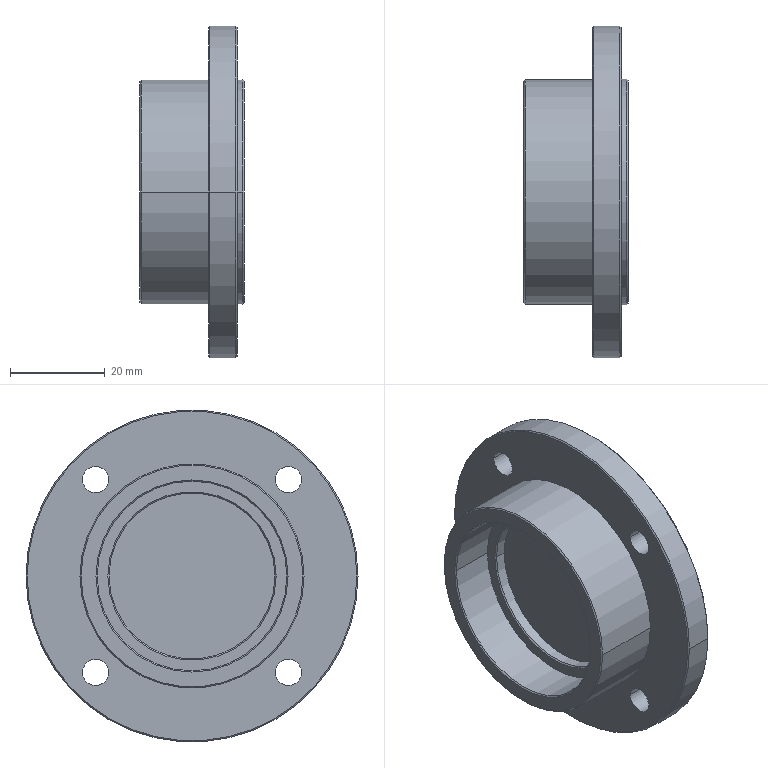Part | STEP file | 2026.6.15-Main Assembly图.sldasm-Part-104 | 1 solid | 36 faces | box 22 x 70 x 70 mm | volume 36230 mm3 | cylinder 18 | cone 12 | plane 6 | commonest cylinder face diameters 5.5 x8 35 x2 40 x2 47.25 x2 47.5 x2 70 x2
STEP:
#1=CARTESIAN_POINT('',(-1505.974,579.301,4296.167));
#2=VERTEX_POINT('',#1);
#3=CARTESIAN_POINT('',(-1505.974,539.301,4296.167));
#4=VERTEX_POINT('',#3);
#5=CARTESIAN_POINT('',(-1505.974,559.301,4296.167));
#6=DIRECTION('',(-1.,0.,0.));
#7=DIRECTION('',(0.,1.,0.));
#8=AXIS2_PLACEMENT_3D('',#5,#6,#7);
#9=CIRCLE('',#8,20.);
#10=EDGE_CURVE('',#2,#4,#9,.T.);
#11=ORIENTED_EDGE('',*,*,#10,.F.);
#12=CARTESIAN_POINT('',(-1506.224,579.551,4296.167));
#13=VERTEX_POINT('',#12);
#14=CARTESIAN_POINT('',(-1506.224,579.551,4296.167));
#15=DIRECTION('',(-0.7071,0.7071,0.));
#16=VECTOR('',#15,1000.);
#17=LINE('',#14,#16);
#18=EDGE_CURVE('',#2,#13,#17,.T.);
#19=ORIENTED_EDGE('',*,*,#18,.T.);
#20=CARTESIAN_POINT('',(-1506.224,539.051,4296.167));
#21=VERTEX_POINT('',#20);
#22=CARTESIAN_POINT('',(-1506.224,559.301,4296.167));
#23=DIRECTION('',(1.,0.,0.));
#24=DIRECTION('',(0.,0.,-1.));
#25=AXIS2_PLACEMENT_3D('',#22,#23,#24);
#26=CIRCLE('',#25,20.25);
#27=EDGE_CURVE('',#21,#13,#26,.T.);
#28=ORIENTED_EDGE('',*,*,#27,.F.);
#29=CARTESIAN_POINT('',(-1506.224,539.051,4296.167));
#30=DIRECTION('',(-0.7071,-0.7071,0.));
#31=VECTOR('',#30,1000.);
#32=LINE('',#29,#31);
#33=EDGE_CURVE('',#4,#21,#32,.T.);
#34=ORIENTED_EDGE('',*,*,#33,.F.);
#35=EDGE_LOOP('',(#11,#19,#28,#34));
#36=FACE_OUTER_BOUND('',#35,.T.);
#37=CARTESIAN_POINT('',(-1506.224,559.301,4296.167));
#38=DIRECTION('',(-1.,0.,0.));
#39=DIRECTION('',(0.,-1.,0.));
#40=AXIS2_PLACEMENT_3D('',#37,#38,#39);
#41=CONICAL_SURFACE('',#40,20.25,0.7854);
#42=ADVANCED_FACE('',(#36),#41,.F.);
#43=CARTESIAN_POINT('',(-1506.224,535.926,4296.167));
#44=VERTEX_POINT('',#43);
#45=CARTESIAN_POINT('',(-1506.224,582.676,4296.167));
#46=VERTEX_POINT('',#45);
#47=CARTESIAN_POINT('',(-1506.224,559.301,4296.167));
#48=DIRECTION('',(-1.,0.,0.));
#49=DIRECTION('',(0.,0.,-1.));
#50=AXIS2_PLACEMENT_3D('',#47,#48,#49);
#51=CIRCLE('',#50,23.375);
#52=EDGE_CURVE('',#44,#46,#51,.T.);
#53=ORIENTED_EDGE('',*,*,#52,.F.);
#54=CARTESIAN_POINT('',(-1505.974,535.676,4296.167));
#55=VERTEX_POINT('',#54);
#56=CARTESIAN_POINT('',(-1505.974,535.676,4296.167));
#57=DIRECTION('',(0.7071,-0.7071,0.));
#58=VECTOR('',#57,1000.);
#59=LINE('',#56,#58);
#60=EDGE_CURVE('',#44,#55,#59,.T.);
#61=ORIENTED_EDGE('',*,*,#60,.T.);
#62=CARTESIAN_POINT('',(-1505.974,582.926,4296.167));
#63=VERTEX_POINT('',#62);
#64=CARTESIAN_POINT('',(-1505.974,559.301,4296.167));
#65=DIRECTION('',(1.,0.,0.));
#66=DIRECTION('',(0.,1.,0.));
#67=AXIS2_PLACEMENT_3D('',#64,#65,#66);
#68=CIRCLE('',#67,23.625);
#69=EDGE_CURVE('',#63,#55,#68,.T.);
#70=ORIENTED_EDGE('',*,*,#69,.F.);
#71=CARTESIAN_POINT('',(-1505.974,582.926,4296.167));
#72=DIRECTION('',(0.7071,0.7071,0.));
#73=VECTOR('',#72,1000.);
#74=LINE('',#71,#73);
#75=EDGE_CURVE('',#46,#63,#74,.T.);
#76=ORIENTED_EDGE('',*,*,#75,.F.);
#77=EDGE_LOOP('',(#53,#61,#70,#76));
#78=FACE_OUTER_BOUND('',#77,.T.);
#79=CARTESIAN_POINT('',(-1505.974,559.301,4296.167));
#80=DIRECTION('',(1.,0.,0.));
#81=DIRECTION('',(0.,1.,0.));
#82=AXIS2_PLACEMENT_3D('',#79,#80,#81);
#83=CONICAL_SURFACE('',#82,23.625,0.7854);
#84=ADVANCED_FACE('',(#78),#83,.T.);
#85=CARTESIAN_POINT('',(-1496.474,576.801,4296.167));
#86=VERTEX_POINT('',#85);
#87=CARTESIAN_POINT('',(-1496.474,541.801,4296.167));
#88=VERTEX_POINT('',#87);
#89=CARTESIAN_POINT('',(-1496.474,559.301,4296.167));
#90=DIRECTION('',(-1.,0.,0.));
#91=DIRECTION('',(0.,1.,0.));
#92=AXIS2_PLACEMENT_3D('',#89,#90,#91);
#93=CIRCLE('',#92,17.5);
#94=EDGE_CURVE('',#86,#88,#93,.T.);
#95=ORIENTED_EDGE('',*,*,#94,.F.);
#96=CARTESIAN_POINT('',(-1496.724,577.051,4296.167));
#97=VERTEX_POINT('',#96);
#98=CARTESIAN_POINT('',(-1496.724,577.051,4296.167));
#99=DIRECTION('',(-0.7071,0.7071,0.));
#100=VECTOR('',#99,1000.);
#101=LINE('',#98,#100);
#102=EDGE_CURVE('',#86,#97,#101,.T.);
#103=ORIENTED_EDGE('',*,*,#102,.T.);
#104=CARTESIAN_POINT('',(-1496.724,541.551,4296.167));
#105=VERTEX_POINT('',#104);
#106=CARTESIAN_POINT('',(-1496.724,559.301,4296.167));
#107=DIRECTION('',(1.,0.,0.));
#108=DIRECTION('',(0.,0.,-1.));
#109=AXIS2_PLACEMENT_3D('',#106,#107,#108);
#110=CIRCLE('',#109,17.75);
#111=EDGE_CURVE('',#105,#97,#110,.T.);
#112=ORIENTED_EDGE('',*,*,#111,.F.);
#113=CARTESIAN_POINT('',(-1496.724,541.551,4296.167));
#114=DIRECTION('',(-0.7071,-0.7071,0.));
#115=VECTOR('',#114,1000.);
#116=LINE('',#113,#115);
#117=EDGE_CURVE('',#88,#105,#116,.T.);
#118=ORIENTED_EDGE('',*,*,#117,.F.);
#119=EDGE_LOOP('',(#95,#103,#112,#118));
#120=FACE_OUTER_BOUND('',#119,.T.);
#121=CARTESIAN_POINT('',(-1496.724,559.301,4296.167));
#122=DIRECTION('',(-1.,0.,0.));
#123=DIRECTION('',(0.,-1.,0.));
#124=AXIS2_PLACEMENT_3D('',#121,#122,#123);
#125=CONICAL_SURFACE('',#124,17.75,0.7854);
#126=ADVANCED_FACE('',(#120),#125,.F.);
#127=CARTESIAN_POINT('',(-1491.724,524.551,4296.167));
#128=VERTEX_POINT('',#127);
#129=CARTESIAN_POINT('',(-1491.724,594.051,4296.167));
#130=VERTEX_POINT('',#129);
#131=CARTESIAN_POINT('',(-1491.724,559.301,4296.167));
#132=DIRECTION('',(-1.,0.,0.));
#133=DIRECTION('',(0.,0.,1.));
#134=AXIS2_PLACEMENT_3D('',#131,#132,#133);
#135=CIRCLE('',#134,34.75);
#136=EDGE_CURVE('',#128,#130,#135,.T.);
#137=ORIENTED_EDGE('',*,*,#136,.F.);
#138=CARTESIAN_POINT('',(-1491.474,524.301,4296.167));
#139=VERTEX_POINT('',#138);
#140=CARTESIAN_POINT('',(-1491.724,524.551,4296.167));
#141=DIRECTION('',(0.7071,-0.7071,0.));
#142=VECTOR('',#141,1000.);
#143=LINE('',#140,#142);
#144=EDGE_CURVE('',#128,#139,#143,.T.);
#145=ORIENTED_EDGE('',*,*,#144,.T.);
#146=CARTESIAN_POINT('',(-1491.474,594.301,4296.167));
#147=VERTEX_POINT('',#146);
#148=CARTESIAN_POINT('',(-1491.474,559.301,4296.167));
#149=DIRECTION('',(1.,0.,0.));
#150=DIRECTION('',(0.,-1.,0.));
#151=AXIS2_PLACEMENT_3D('',#148,#149,#150);
#152=CIRCLE('',#151,35.);
#153=EDGE_CURVE('',#147,#139,#152,.T.);
#154=ORIENTED_EDGE('',*,*,#153,.F.);
#155=CARTESIAN_POINT('',(-1491.724,594.051,4296.167));
#156=DIRECTION('',(0.7071,0.7071,0.));
#157=VECTOR('',#156,1000.);
#158=LINE('',#155,#157);
#159=EDGE_CURVE('',#130,#147,#158,.T.);
#160=ORIENTED_EDGE('',*,*,#159,.F.);
#161=EDGE_LOOP('',(#137,#145,#154,#160));
#162=FACE_OUTER_BOUND('',#161,.T.);
#163=CARTESIAN_POINT('',(-1491.724,559.301,4296.167));
#164=DIRECTION('',(1.,0.,0.));
#165=DIRECTION('',(0.,1.,0.));
#166=AXIS2_PLACEMENT_3D('',#163,#164,#165);
#167=CONICAL_SURFACE('',#166,34.75,0.7854);
#168=ADVANCED_FACE('',(#162),#167,.T.);
#169=CARTESIAN_POINT('',(-1485.724,594.051,4296.167));
#170=VERTEX_POINT('',#169);
#171=CARTESIAN_POINT('',(-1485.724,524.551,4296.167));
#172=VERTEX_POINT('',#171);
#173=CARTESIAN_POINT('',(-1485.724,559.301,4296.167));
#174=DIRECTION('',(1.,0.,0.));
#175=DIRECTION('',(0.,0.,1.));
#176=AXIS2_PLACEMENT_3D('',#173,#174,#175);
#177=CIRCLE('',#176,34.75);
#178=EDGE_CURVE('',#170,#172,#177,.T.);
#179=ORIENTED_EDGE('',*,*,#178,.F.);
#180=CARTESIAN_POINT('',(-1485.974,594.301,4296.167));
#181=VERTEX_POINT('',#180);
#182=CARTESIAN_POINT('',(-1485.974,594.301,4296.167));
#183=DIRECTION('',(-0.7071,0.7071,0.));
#184=VECTOR('',#183,1000.);
#185=LINE('',#182,#184);
#186=EDGE_CURVE('',#170,#181,#185,.T.);
#187=ORIENTED_EDGE('',*,*,#186,.T.);
#188=CARTESIAN_POINT('',(-1485.974,524.301,4296.167));
#189=VERTEX_POINT('',#188);
#190=CARTESIAN_POINT('',(-1485.974,559.301,4296.167));
#191=DIRECTION('',(-1.,0.,0.));
#192=DIRECTION('',(0.,-1.,0.));
#193=AXIS2_PLACEMENT_3D('',#190,#191,#192);
#194=CIRCLE('',#193,35.);
#195=EDGE_CURVE('',#189,#181,#194,.T.);
#196=ORIENTED_EDGE('',*,*,#195,.F.);
#197=CARTESIAN_POINT('',(-1485.974,524.301,4296.167));
#198=DIRECTION('',(-0.7071,-0.7071,0.));
#199=VECTOR('',#198,1000.);
#200=LINE('',#197,#199);
#201=EDGE_CURVE('',#172,#189,#200,.T.);
#202=ORIENTED_EDGE('',*,*,#201,.F.);
#203=EDGE_LOOP('',(#179,#187,#196,#202));
#204=FACE_OUTER_BOUND('',#203,.T.);
#205=CARTESIAN_POINT('',(-1485.974,559.301,4296.167));
#206=DIRECTION('',(-1.,0.,0.));
#207=DIRECTION('',(0.,-1.,0.));
#208=AXIS2_PLACEMENT_3D('',#205,#206,#207);
#209=CONICAL_SURFACE('',#208,35.,0.7854);
#210=ADVANCED_FACE('',(#204),#209,.T.);
#211=CARTESIAN_POINT('',(-1484.224,582.801,4296.167));
#212=VERTEX_POINT('',#211);
#213=CARTESIAN_POINT('',(-1484.224,535.801,4296.167));
#214=VERTEX_POINT('',#213);
#215=CARTESIAN_POINT('',(-1484.224,559.301,4296.167));
#216=DIRECTION('',(1.,0.,0.));
#217=DIRECTION('',(0.,0.,1.));
#218=AXIS2_PLACEMENT_3D('',#215,#216,#217);
#219=CIRCLE('',#218,23.5);
#220=EDGE_CURVE('',#212,#214,#219,.T.);
#221=ORIENTED_EDGE('',*,*,#220,.F.);
#222=CARTESIAN_POINT('',(-1484.474,583.051,4296.167));
#223=VERTEX_POINT('',#222);
#224=CARTESIAN_POINT('',(-1484.224,582.801,4296.167));
#225=DIRECTION('',(-0.7071,0.7071,0.));
#226=VECTOR('',#225,1000.);
#227=LINE('',#224,#226);
#228=EDGE_CURVE('',#212,#223,#227,.T.);
#229=ORIENTED_EDGE('',*,*,#228,.T.);
#230=CARTESIAN_POINT('',(-1484.474,535.551,4296.167));
#231=VERTEX_POINT('',#230);
#232=CARTESIAN_POINT('',(-1484.474,559.301,4296.167));
#233=DIRECTION('',(-1.,0.,0.));
#234=DIRECTION('',(0.,-1.,0.));
#235=AXIS2_PLACEMENT_3D('',#232,#233,#234);
#236=CIRCLE('',#235,23.75);
#237=EDGE_CURVE('',#231,#223,#236,.T.);
#238=ORIENTED_EDGE('',*,*,#237,.F.);
#239=CARTESIAN_POINT('',(-1484.224,535.801,4296.167));
#240=DIRECTION('',(-0.7071,-0.7071,0.));
#241=VECTOR('',#240,1000.);
#242=LINE('',#239,#241);
#243=EDGE_CURVE('',#214,#231,#242,.T.);
#244=ORIENTED_EDGE('',*,*,#243,.F.);
#245=EDGE_LOOP('',(#221,#229,#238,#244));
#246=FACE_OUTER_BOUND('',#245,.T.);
#247=CARTESIAN_POINT('',(-1484.224,559.301,4296.167));
#248=DIRECTION('',(-1.,0.,0.));
#249=DIRECTION('',(0.,-1.,0.));
#250=AXIS2_PLACEMENT_3D('',#247,#248,#249);
#251=CONICAL_SURFACE('',#250,23.5,0.7854);
#252=ADVANCED_FACE('',(#246),#251,.T.);
#253=ORIENTED_EDGE('',*,*,#237,.T.);
#254=CARTESIAN_POINT('',(-1485.724,583.051,4296.167));
#255=VERTEX_POINT('',#254);
#256=CARTESIAN_POINT('',(-1484.224,583.051,4296.167));
#257=DIRECTION('',(-1.,0.,0.));
#258=VECTOR('',#257,1000.);
#259=LINE('',#256,#258);
#260=EDGE_CURVE('',#223,#255,#259,.T.);
#261=ORIENTED_EDGE('',*,*,#260,.T.);
#262=CARTESIAN_POINT('',(-1485.724,535.551,4296.167));
#263=VERTEX_POINT('',#262);
#264=CARTESIAN_POINT('',(-1485.724,559.301,4296.167));
#265=DIRECTION('',(1.,0.,0.));
#266=DIRECTION('',(0.,0.7071,0.7071));
#267=AXIS2_PLACEMENT_3D('',#264,#265,#266);
#268=CIRCLE('',#267,23.75);
#269=EDGE_CURVE('',#255,#263,#268,.T.);
#270=ORIENTED_EDGE('',*,*,#269,.T.);
#271=CARTESIAN_POINT('',(-1484.224,535.551,4296.167));
#272=DIRECTION('',(-1.,0.,0.));
#273=VECTOR('',#272,1000.);
#274=LINE('',#271,#273);
#275=EDGE_CURVE('',#231,#263,#274,.T.);
#276=ORIENTED_EDGE('',*,*,#275,.F.);
#277=EDGE_LOOP('',(#253,#261,#270,#276));
#278=FACE_OUTER_BOUND('',#277,.T.);
#279=CARTESIAN_POINT('',(-1484.224,559.301,4296.167));
#280=DIRECTION('',(-1.,0.,0.));
#281=DIRECTION('',(0.,-1.,0.));
#282=AXIS2_PLACEMENT_3D('',#279,#280,#281);
#283=CYLINDRICAL_SURFACE('',#282,23.75);
#284=ADVANCED_FACE('',(#278),#283,.T.);
#285=CARTESIAN_POINT('',(-1494.224,541.801,4296.167));
#286=VERTEX_POINT('',#285);
#287=CARTESIAN_POINT('',(-1494.224,576.801,4296.167));
#288=VERTEX_POINT('',#287);
#289=CARTESIAN_POINT('',(-1494.224,559.301,4296.167));
#290=DIRECTION('',(1.,0.,0.));
#291=DIRECTION('',(0.,-0.7071,0.7071));
#292=AXIS2_PLACEMENT_3D('',#289,#290,#291);
#293=CIRCLE('',#292,17.5);
#294=EDGE_CURVE('',#286,#288,#293,.T.);
#295=ORIENTED_EDGE('',*,*,#294,.T.);
#296=CARTESIAN_POINT('',(-1494.224,576.801,4296.167));
#297=DIRECTION('',(-1.,0.,0.));
#298=VECTOR('',#297,1000.);
#299=LINE('',#296,#298);
#300=EDGE_CURVE('',#288,#86,#299,.T.);
#301=ORIENTED_EDGE('',*,*,#300,.T.);
#302=ORIENTED_EDGE('',*,*,#94,.T.);
#303=CARTESIAN_POINT('',(-1494.224,541.801,4296.167));
#304=DIRECTION('',(-1.,0.,0.));
#305=VECTOR('',#304,1000.);
#306=LINE('',#303,#305);
#307=EDGE_CURVE('',#286,#88,#306,.T.);
#308=ORIENTED_EDGE('',*,*,#307,.F.);
#309=EDGE_LOOP('',(#295,#301,#302,#308));
#310=FACE_OUTER_BOUND('',#309,.T.);
#311=CARTESIAN_POINT('',(-1494.224,559.301,4296.167));
#312=DIRECTION('',(-1.,0.,0.));
#313=DIRECTION('',(0.,-1.,0.));
#314=AXIS2_PLACEMENT_3D('',#311,#312,#313);
#315=CYLINDRICAL_SURFACE('',#314,17.5);
#316=ADVANCED_FACE('',(#310),#315,.F.);
#317=CARTESIAN_POINT('',(-1496.724,579.301,4296.167));
#318=VERTEX_POINT('',#317);
#319=CARTESIAN_POINT('',(-1496.724,539.301,4296.167));
#320=VERTEX_POINT('',#319);
#321=CARTESIAN_POINT('',(-1496.724,559.301,4296.167));
#322=DIRECTION('',(-1.,0.,0.));
#323=DIRECTION('',(0.,-0.7071,-0.7071));
#324=AXIS2_PLACEMENT_3D('',#321,#322,#323);
#325=CIRCLE('',#324,20.);
#326=EDGE_CURVE('',#318,#320,#325,.T.);
#327=ORIENTED_EDGE('',*,*,#326,.F.);
#328=CARTESIAN_POINT('',(-1496.724,579.301,4296.167));
#329=DIRECTION('',(-1.,0.,0.));
#330=VECTOR('',#329,1000.);
#331=LINE('',#328,#330);
#332=EDGE_CURVE('',#318,#2,#331,.T.);
#333=ORIENTED_EDGE('',*,*,#332,.T.);
#334=ORIENTED_EDGE('',*,*,#10,.T.);
#335=CARTESIAN_POINT('',(-1496.724,539.301,4296.167));
#336=DIRECTION('',(-1.,0.,0.));
#337=VECTOR('',#336,1000.);
#338=LINE('',#335,#337);
#339=EDGE_CURVE('',#320,#4,#338,.T.);
#340=ORIENTED_EDGE('',*,*,#339,.F.);
#341=EDGE_LOOP('',(#327,#333,#334,#340));
#342=FACE_OUTER_BOUND('',#341,.T.);
#343=CARTESIAN_POINT('',(-1496.724,559.301,4296.167));
#344=DIRECTION('',(-1.,0.,0.));
#345=DIRECTION('',(0.,-1.,0.));
#346=AXIS2_PLACEMENT_3D('',#343,#344,#345);
#347=CYLINDRICAL_SURFACE('',#346,20.);
#348=ADVANCED_FACE('',(#342),#347,.F.);
#349=CARTESIAN_POINT('',(-1485.724,536.222,4275.837));
#350=VERTEX_POINT('',#349);
#351=CARTESIAN_POINT('',(-1485.724,541.722,4275.837));
#352=VERTEX_POINT('',#351);
#353=CARTESIAN_POINT('',(-1485.724,538.972,4275.837));
#354=DIRECTION('',(1.,0.,0.));
#355=DIRECTION('',(0.,0.7071,0.7071));
#356=AXIS2_PLACEMENT_3D('',#353,#354,#355);
#357=CIRCLE('',#356,2.75);
#358=EDGE_CURVE('',#350,#352,#357,.T.);
#359=ORIENTED_EDGE('',*,*,#358,.T.);
#360=CARTESIAN_POINT('',(-1491.724,541.722,4275.837));
#361=VERTEX_POINT('',#360);
#362=CARTESIAN_POINT('',(-1485.724,541.722,4275.837));
#363=DIRECTION('',(-1.,0.,0.));
#364=VECTOR('',#363,1000.);
#365=LINE('',#362,#364);
#366=EDGE_CURVE('',#352,#361,#365,.T.);
#367=ORIENTED_EDGE('',*,*,#366,.T.);
#368=CARTESIAN_POINT('',(-1491.724,536.222,4275.837));
#369=VERTEX_POINT('',#368);
#370=CARTESIAN_POINT('',(-1491.724,538.972,4275.837));
#371=DIRECTION('',(1.,0.,0.));
#372=DIRECTION('',(0.,0.7071,0.7071));
#373=AXIS2_PLACEMENT_3D('',#370,#371,#372);
#374=CIRCLE('',#373,2.75);
#375=EDGE_CURVE('',#369,#361,#374,.T.);
#376=ORIENTED_EDGE('',*,*,#375,.F.);
#377=CARTESIAN_POINT('',(-1485.724,536.222,4275.837));
#378=DIRECTION('',(-1.,0.,0.));
#379=VECTOR('',#378,1000.);
#380=LINE('',#377,#379);
#381=EDGE_CURVE('',#350,#369,#380,.T.);
#382=ORIENTED_EDGE('',*,*,#381,.F.);
#383=EDGE_LOOP('',(#359,#367,#376,#382));
#384=FACE_OUTER_BOUND('',#383,.T.);
#385=CARTESIAN_POINT('',(-1485.724,538.972,4275.837));
#386=DIRECTION('',(-1.,0.,0.));
#387=DIRECTION('',(0.,-1.,0.));
#388=AXIS2_PLACEMENT_3D('',#385,#386,#387);
#389=CYLINDRICAL_SURFACE('',#388,2.75);
#390=ADVANCED_FACE('',(#384),#389,.F.);
#391=ORIENTED_EDGE('',*,*,#195,.T.);
#392=CARTESIAN_POINT('',(-1485.724,594.301,4296.167));
#393=DIRECTION('',(-1.,0.,0.));
#394=VECTOR('',#393,1000.);
#395=LINE('',#392,#394);
#396=EDGE_CURVE('',#181,#147,#395,.T.);
#397=ORIENTED_EDGE('',*,*,#396,.T.);
#398=ORIENTED_EDGE('',*,*,#153,.T.);
#399=CARTESIAN_POINT('',(-1485.724,524.301,4296.167));
#400=DIRECTION('',(-1.,0.,0.));
#401=VECTOR('',#400,1000.);
#402=LINE('',#399,#401);
#403=EDGE_CURVE('',#189,#139,#402,.T.);
#404=ORIENTED_EDGE('',*,*,#403,.F.);
#405=EDGE_LOOP('',(#391,#397,#398,#404));
#406=FACE_OUTER_BOUND('',#405,.T.);
#407=CARTESIAN_POINT('',(-1485.724,559.301,4296.167));
#408=DIRECTION('',(-1.,0.,0.));
#409=DIRECTION('',(0.,-1.,0.));
#410=AXIS2_PLACEMENT_3D('',#407,#408,#409);
#411=CYLINDRICAL_SURFACE('',#410,35.);
#412=ADVANCED_FACE('',(#406),#411,.T.);
#413=CARTESIAN_POINT('',(-1485.724,576.881,4316.496));
#414=VERTEX_POINT('',#413);
#415=CARTESIAN_POINT('',(-1485.724,582.381,4316.496));
#416=VERTEX_POINT('',#415);
#417=CARTESIAN_POINT('',(-1485.724,579.631,4316.496));
#418=DIRECTION('',(1.,0.,0.));
#419=DIRECTION('',(0.,0.7071,0.7071));
#420=AXIS2_PLACEMENT_3D('',#417,#418,#419);
#421=CIRCLE('',#420,2.75);
#422=EDGE_CURVE('',#414,#416,#421,.T.);
#423=ORIENTED_EDGE('',*,*,#422,.T.);
#424=CARTESIAN_POINT('',(-1491.724,582.381,4316.496));
#425=VERTEX_POINT('',#424);
#426=CARTESIAN_POINT('',(-1485.724,582.381,4316.496));
#427=DIRECTION('',(-1.,0.,0.));
#428=VECTOR('',#427,1000.);
#429=LINE('',#426,#428);
#430=EDGE_CURVE('',#416,#425,#429,.T.);
#431=ORIENTED_EDGE('',*,*,#430,.T.);
#432=CARTESIAN_POINT('',(-1491.724,576.881,4316.496));
#433=VERTEX_POINT('',#432);
#434=CARTESIAN_POINT('',(-1491.724,579.631,4316.496));
#435=DIRECTION('',(1.,0.,0.));
#436=DIRECTION('',(0.,0.7071,0.7071));
#437=AXIS2_PLACEMENT_3D('',#434,#435,#436);
#438=CIRCLE('',#437,2.75);
#439=EDGE_CURVE('',#433,#425,#438,.T.);
#440=ORIENTED_EDGE('',*,*,#439,.F.);
#441=CARTESIAN_POINT('',(-1485.724,576.881,4316.496));
#442=DIRECTION('',(-1.,0.,0.));
#443=VECTOR('',#442,1000.);
#444=LINE('',#441,#443);
#445=EDGE_CURVE('',#414,#433,#444,.T.);
#446=ORIENTED_EDGE('',*,*,#445,.F.);
#447=EDGE_LOOP('',(#423,#431,#440,#446));
#448=FACE_OUTER_BOUND('',#447,.T.);
#449=CARTESIAN_POINT('',(-1485.724,579.631,4316.496));
#450=DIRECTION('',(-1.,0.,0.));
#451=DIRECTION('',(0.,-1.,0.));
#452=AXIS2_PLACEMENT_3D('',#449,#450,#451);
#453=CYLINDRICAL_SURFACE('',#452,2.75);
#454=ADVANCED_FACE('',(#448),#453,.F.);
#455=CARTESIAN_POINT('',(-1485.724,536.222,4316.496));
#456=VERTEX_POINT('',#455);
#457=CARTESIAN_POINT('',(-1485.724,541.722,4316.496));
#458=VERTEX_POINT('',#457);
#459=CARTESIAN_POINT('',(-1485.724,538.972,4316.496));
#460=DIRECTION('',(1.,0.,0.));
#461=DIRECTION('',(0.,0.7071,0.7071));
#462=AXIS2_PLACEMENT_3D('',#459,#460,#461);
#463=CIRCLE('',#462,2.75);
#464=EDGE_CURVE('',#456,#458,#463,.T.);
#465=ORIENTED_EDGE('',*,*,#464,.T.);
#466=CARTESIAN_POINT('',(-1491.724,541.722,4316.496));
#467=VERTEX_POINT('',#466);
#468=CARTESIAN_POINT('',(-1485.724,541.722,4316.496));
#469=DIRECTION('',(-1.,0.,0.));
#470=VECTOR('',#469,1000.);
#471=LINE('',#468,#470);
#472=EDGE_CURVE('',#458,#467,#471,.T.);
#473=ORIENTED_EDGE('',*,*,#472,.T.);
#474=CARTESIAN_POINT('',(-1491.724,536.222,4316.496));
#475=VERTEX_POINT('',#474);
#476=CARTESIAN_POINT('',(-1491.724,538.972,4316.496));
#477=DIRECTION('',(1.,0.,0.));
#478=DIRECTION('',(0.,0.7071,0.7071));
#479=AXIS2_PLACEMENT_3D('',#476,#477,#478);
#480=CIRCLE('',#479,2.75);
#481=EDGE_CURVE('',#475,#467,#480,.T.);
#482=ORIENTED_EDGE('',*,*,#481,.F.);
#483=CARTESIAN_POINT('',(-1485.724,536.222,4316.496));
#484=DIRECTION('',(-1.,0.,0.));
#485=VECTOR('',#484,1000.);
#486=LINE('',#483,#485);
#487=EDGE_CURVE('',#456,#475,#486,.T.);
#488=ORIENTED_EDGE('',*,*,#487,.F.);
#489=EDGE_LOOP('',(#465,#473,#482,#488));
#490=FACE_OUTER_BOUND('',#489,.T.);
#491=CARTESIAN_POINT('',(-1485.724,538.972,4316.496));
#492=DIRECTION('',(-1.,0.,0.));
#493=DIRECTION('',(0.,-1.,0.));
#494=AXIS2_PLACEMENT_3D('',#491,#492,#493);
#495=CYLINDRICAL_SURFACE('',#494,2.75);
#496=ADVANCED_FACE('',(#490),#495,.F.);
#497=CARTESIAN_POINT('',(-1485.724,576.881,4275.837));
#498=VERTEX_POINT('',#497);
#499=CARTESIAN_POINT('',(-1485.724,582.381,4275.837));
#500=VERTEX_POINT('',#499);
#501=CARTESIAN_POINT('',(-1485.724,579.631,4275.837));
#502=DIRECTION('',(1.,0.,0.));
#503=DIRECTION('',(0.,0.7071,0.7071));
#504=AXIS2_PLACEMENT_3D('',#501,#502,#503);
#505=CIRCLE('',#504,2.75);
#506=EDGE_CURVE('',#498,#500,#505,.T.);
#507=ORIENTED_EDGE('',*,*,#506,.T.);
#508=CARTESIAN_POINT('',(-1491.724,582.381,4275.837));
#509=VERTEX_POINT('',#508);
#510=CARTESIAN_POINT('',(-1485.724,582.381,4275.837));
#511=DIRECTION('',(-1.,0.,0.));
#512=VECTOR('',#511,1000.);
#513=LINE('',#510,#512);
#514=EDGE_CURVE('',#500,#509,#513,.T.);
#515=ORIENTED_EDGE('',*,*,#514,.T.);
#516=CARTESIAN_POINT('',(-1491.724,576.881,4275.837));
#517=VERTEX_POINT('',#516);
#518=CARTESIAN_POINT('',(-1491.724,579.631,4275.837));
#519=DIRECTION('',(1.,0.,0.));
#520=DIRECTION('',(0.,0.7071,0.7071));
#521=AXIS2_PLACEMENT_3D('',#518,#519,#520);
#522=CIRCLE('',#521,2.75);
#523=EDGE_CURVE('',#517,#509,#522,.T.);
#524=ORIENTED_EDGE('',*,*,#523,.F.);
#525=CARTESIAN_POINT('',(-1485.724,576.881,4275.837));
#526=DIRECTION('',(-1.,0.,0.));
#527=VECTOR('',#526,1000.);
#528=LINE('',#525,#527);
#529=EDGE_CURVE('',#498,#517,#528,.T.);
#530=ORIENTED_EDGE('',*,*,#529,.F.);
#531=EDGE_LOOP('',(#507,#515,#524,#530));
#532=FACE_OUTER_BOUND('',#531,.T.);
#533=CARTESIAN_POINT('',(-1485.724,579.631,4275.837));
#534=DIRECTION('',(-1.,0.,0.));
#535=DIRECTION('',(0.,-1.,0.));
#536=AXIS2_PLACEMENT_3D('',#533,#534,#535);
#537=CYLINDRICAL_SURFACE('',#536,2.75);
#538=ADVANCED_FACE('',(#532),#537,.F.);
#539=CARTESIAN_POINT('',(-1491.724,582.926,4296.167));
#540=VERTEX_POINT('',#539);
#541=CARTESIAN_POINT('',(-1491.724,535.676,4296.167));
#542=VERTEX_POINT('',#541);
#543=CARTESIAN_POINT('',(-1491.724,559.301,4296.167));
#544=DIRECTION('',(1.,0.,0.));
#545=DIRECTION('',(0.,-0.7071,-0.7071));
#546=AXIS2_PLACEMENT_3D('',#543,#544,#545);
#547=CIRCLE('',#546,23.625);
#548=EDGE_CURVE('',#540,#542,#547,.T.);
#549=ORIENTED_EDGE('',*,*,#548,.F.);
#550=CARTESIAN_POINT('',(-1491.724,582.926,4296.167));
#551=DIRECTION('',(-1.,0.,0.));
#552=VECTOR('',#551,1000.);
#553=LINE('',#550,#552);
#554=EDGE_CURVE('',#540,#63,#553,.T.);
#555=ORIENTED_EDGE('',*,*,#554,.T.);
#556=ORIENTED_EDGE('',*,*,#69,.T.);
#557=CARTESIAN_POINT('',(-1491.724,535.676,4296.167));
#558=DIRECTION('',(-1.,0.,0.));
#559=VECTOR('',#558,1000.);
#560=LINE('',#557,#559);
#561=EDGE_CURVE('',#542,#55,#560,.T.);
#562=ORIENTED_EDGE('',*,*,#561,.F.);
#563=EDGE_LOOP('',(#549,#555,#556,#562));
#564=FACE_OUTER_BOUND('',#563,.T.);
#565=CARTESIAN_POINT('',(-1491.724,559.301,4296.167));
#566=DIRECTION('',(-1.,0.,0.));
#567=DIRECTION('',(0.,-1.,0.));
#568=AXIS2_PLACEMENT_3D('',#565,#566,#567);
#569=CYLINDRICAL_SURFACE('',#568,23.625);
#570=ADVANCED_FACE('',(#564),#569,.T.);
#571=ORIENTED_EDGE('',*,*,#554,.F.);
#572=CARTESIAN_POINT('',(-1491.724,559.301,4296.167));
#573=DIRECTION('',(1.,0.,0.));
#574=DIRECTION('',(0.,-0.7071,-0.7071));
#575=AXIS2_PLACEMENT_3D('',#572,#573,#574);
#576=CIRCLE('',#575,23.625);
#577=EDGE_CURVE('',#542,#540,#576,.T.);
#578=ORIENTED_EDGE('',*,*,#577,.F.);
#579=ORIENTED_EDGE('',*,*,#561,.T.);
#580=CARTESIAN_POINT('',(-1505.974,559.301,4296.167));
#581=DIRECTION('',(1.,0.,0.));
#582=DIRECTION('',(0.,1.,0.));
#583=AXIS2_PLACEMENT_3D('',#580,#581,#582);
#584=CIRCLE('',#583,23.625);
#585=EDGE_CURVE('',#55,#63,#584,.T.);
#586=ORIENTED_EDGE('',*,*,#585,.T.);
#587=EDGE_LOOP('',(#571,#578,#579,#586));
#588=FACE_OUTER_BOUND('',#587,.T.);
#589=CARTESIAN_POINT('',(-1491.724,559.301,4296.167));
#590=DIRECTION('',(-1.,0.,0.));
#591=DIRECTION('',(0.,-1.,0.));
#592=AXIS2_PLACEMENT_3D('',#589,#590,#591);
#593=CYLINDRICAL_SURFACE('',#592,23.625);
#594=ADVANCED_FACE('',(#588),#593,.T.);
#595=CARTESIAN_POINT('',(-1506.224,559.301,4296.167));
#596=DIRECTION('',(-1.,0.,0.));
#597=DIRECTION('',(0.,0.,-1.));
#598=AXIS2_PLACEMENT_3D('',#595,#596,#597);
#599=CIRCLE('',#598,23.375);
#600=EDGE_CURVE('',#46,#44,#599,.T.);
#601=ORIENTED_EDGE('',*,*,#600,.T.);
#602=ORIENTED_EDGE('',*,*,#52,.T.);
#603=EDGE_LOOP('',(#601,#602));
#604=FACE_OUTER_BOUND('',#603,.T.);
#605=ORIENTED_EDGE('',*,*,#27,.T.);
#606=CARTESIAN_POINT('',(-1506.224,559.301,4296.167));
#607=DIRECTION('',(1.,0.,0.));
#608=DIRECTION('',(0.,0.,-1.));
#609=AXIS2_PLACEMENT_3D('',#606,#607,#608);
#610=CIRCLE('',#609,20.25);
#611=EDGE_CURVE('',#13,#21,#610,.T.);
#612=ORIENTED_EDGE('',*,*,#611,.T.);
#613=EDGE_LOOP('',(#605,#612));
#614=FACE_BOUND('',#613,.T.);
#615=CARTESIAN_POINT('',(-1506.224,559.301,4296.167));
#616=DIRECTION('',(1.,0.,0.));
#617=DIRECTION('',(0.,0.,-1.));
#618=AXIS2_PLACEMENT_3D('',#615,#616,#617);
#619=PLANE('',#618);
#620=ADVANCED_FACE('',(#604,#614),#619,.F.);
#621=ORIENTED_EDGE('',*,*,#514,.F.);
#622=CARTESIAN_POINT('',(-1485.724,579.631,4275.837));
#623=DIRECTION('',(1.,0.,0.));
#624=DIRECTION('',(0.,0.7071,0.7071));
#625=AXIS2_PLACEMENT_3D('',#622,#623,#624);
#626=CIRCLE('',#625,2.75);
#627=EDGE_CURVE('',#500,#498,#626,.T.);
#628=ORIENTED_EDGE('',*,*,#627,.T.);
#629=ORIENTED_EDGE('',*,*,#529,.T.);
#630=CARTESIAN_POINT('',(-1491.724,579.631,4275.837));
#631=DIRECTION('',(1.,0.,0.));
#632=DIRECTION('',(0.,0.7071,0.7071));
#633=AXIS2_PLACEMENT_3D('',#630,#631,#632);
#634=CIRCLE('',#633,2.75);
#635=EDGE_CURVE('',#509,#517,#634,.T.);
#636=ORIENTED_EDGE('',*,*,#635,.F.);
#637=EDGE_LOOP('',(#621,#628,#629,#636));
#638=FACE_OUTER_BOUND('',#637,.T.);
#639=CARTESIAN_POINT('',(-1485.724,579.631,4275.837));
#640=DIRECTION('',(-1.,0.,0.));
#641=DIRECTION('',(0.,-1.,0.));
#642=AXIS2_PLACEMENT_3D('',#639,#640,#641);
#643=CYLINDRICAL_SURFACE('',#642,2.75);
#644=ADVANCED_FACE('',(#638),#643,.F.);
#645=ORIENTED_EDGE('',*,*,#472,.F.);
#646=CARTESIAN_POINT('',(-1485.724,538.972,4316.496));
#647=DIRECTION('',(1.,0.,0.));
#648=DIRECTION('',(0.,0.7071,0.7071));
#649=AXIS2_PLACEMENT_3D('',#646,#647,#648);
#650=CIRCLE('',#649,2.75);
#651=EDGE_CURVE('',#458,#456,#650,.T.);
#652=ORIENTED_EDGE('',*,*,#651,.T.);
#653=ORIENTED_EDGE('',*,*,#487,.T.);
#654=CARTESIAN_POINT('',(-1491.724,538.972,4316.496));
#655=DIRECTION('',(1.,0.,0.));
#656=DIRECTION('',(0.,0.7071,0.7071));
#657=AXIS2_PLACEMENT_3D('',#654,#655,#656);
#658=CIRCLE('',#657,2.75);
#659=EDGE_CURVE('',#467,#475,#658,.T.);
#660=ORIENTED_EDGE('',*,*,#659,.F.);
#661=EDGE_LOOP('',(#645,#652,#653,#660));
#662=FACE_OUTER_BOUND('',#661,.T.);
#663=CARTESIAN_POINT('',(-1485.724,538.972,4316.496));
#664=DIRECTION('',(-1.,0.,0.));
#665=DIRECTION('',(0.,-1.,0.));
#666=AXIS2_PLACEMENT_3D('',#663,#664,#665);
#667=CYLINDRICAL_SURFACE('',#666,2.75);
#668=ADVANCED_FACE('',(#662),#667,.F.);
#669=ORIENTED_EDGE('',*,*,#430,.F.);
#670=CARTESIAN_POINT('',(-1485.724,579.631,4316.496));
#671=DIRECTION('',(1.,0.,0.));
#672=DIRECTION('',(0.,0.7071,0.7071));
#673=AXIS2_PLACEMENT_3D('',#670,#671,#672);
#674=CIRCLE('',#673,2.75);
#675=EDGE_CURVE('',#416,#414,#674,.T.);
#676=ORIENTED_EDGE('',*,*,#675,.T.);
#677=ORIENTED_EDGE('',*,*,#445,.T.);
#678=CARTESIAN_POINT('',(-1491.724,579.631,4316.496));
#679=DIRECTION('',(1.,0.,0.));
#680=DIRECTION('',(0.,0.7071,0.7071));
#681=AXIS2_PLACEMENT_3D('',#678,#679,#680);
#682=CIRCLE('',#681,2.75);
#683=EDGE_CURVE('',#425,#433,#682,.T.);
#684=ORIENTED_EDGE('',*,*,#683,.F.);
#685=EDGE_LOOP('',(#669,#676,#677,#684));
#686=FACE_OUTER_BOUND('',#685,.T.);
#687=CARTESIAN_POINT('',(-1485.724,579.631,4316.496));
#688=DIRECTION('',(-1.,0.,0.));
#689=DIRECTION('',(0.,-1.,0.));
#690=AXIS2_PLACEMENT_3D('',#687,#688,#689);
#691=CYLINDRICAL_SURFACE('',#690,2.75);
#692=ADVANCED_FACE('',(#686),#691,.F.);
#693=ORIENTED_EDGE('',*,*,#396,.F.);
#694=CARTESIAN_POINT('',(-1485.974,559.301,4296.167));
#695=DIRECTION('',(-1.,0.,0.));
#696=DIRECTION('',(0.,-1.,0.));
#697=AXIS2_PLACEMENT_3D('',#694,#695,#696);
#698=CIRCLE('',#697,35.);
#699=EDGE_CURVE('',#181,#189,#698,.T.);
#700=ORIENTED_EDGE('',*,*,#699,.T.);
#701=ORIENTED_EDGE('',*,*,#403,.T.);
#702=CARTESIAN_POINT('',(-1491.474,559.301,4296.167));
#703=DIRECTION('',(1.,0.,0.));
#704=DIRECTION('',(0.,-1.,0.));
#705=AXIS2_PLACEMENT_3D('',#702,#703,#704);
#706=CIRCLE('',#705,35.);
#707=EDGE_CURVE('',#139,#147,#706,.T.);
#708=ORIENTED_EDGE('',*,*,#707,.T.);
#709=EDGE_LOOP('',(#693,#700,#701,#708));
#710=FACE_OUTER_BOUND('',#709,.T.);
#711=CARTESIAN_POINT('',(-1485.724,559.301,4296.167));
#712=DIRECTION('',(-1.,0.,0.));
#713=DIRECTION('',(0.,-1.,0.));
#714=AXIS2_PLACEMENT_3D('',#711,#712,#713);
#715=CYLINDRICAL_SURFACE('',#714,35.);
#716=ADVANCED_FACE('',(#710),#715,.T.);
#717=ORIENTED_EDGE('',*,*,#366,.F.);
#718=CARTESIAN_POINT('',(-1485.724,538.972,4275.837));
#719=DIRECTION('',(1.,0.,0.));
#720=DIRECTION('',(0.,0.7071,0.7071));
#721=AXIS2_PLACEMENT_3D('',#718,#719,#720);
#722=CIRCLE('',#721,2.75);
#723=EDGE_CURVE('',#352,#350,#722,.T.);
#724=ORIENTED_EDGE('',*,*,#723,.T.);
#725=ORIENTED_EDGE('',*,*,#381,.T.);
#726=CARTESIAN_POINT('',(-1491.724,538.972,4275.837));
#727=DIRECTION('',(1.,0.,0.));
#728=DIRECTION('',(0.,0.7071,0.7071));
#729=AXIS2_PLACEMENT_3D('',#726,#727,#728);
#730=CIRCLE('',#729,2.75);
#731=EDGE_CURVE('',#361,#369,#730,.T.);
#732=ORIENTED_EDGE('',*,*,#731,.F.);
#733=EDGE_LOOP('',(#717,#724,#725,#732));
#734=FACE_OUTER_BOUND('',#733,.T.);
#735=CARTESIAN_POINT('',(-1485.724,538.972,4275.837));
#736=DIRECTION('',(-1.,0.,0.));
#737=DIRECTION('',(0.,-1.,0.));
#738=AXIS2_PLACEMENT_3D('',#735,#736,#737);
#739=CYLINDRICAL_SURFACE('',#738,2.75);
#740=ADVANCED_FACE('',(#734),#739,.F.);
#741=CARTESIAN_POINT('',(-1485.724,559.301,4296.167));
#742=DIRECTION('',(1.,0.,0.));
#743=DIRECTION('',(0.,0.,1.));
#744=AXIS2_PLACEMENT_3D('',#741,#742,#743);
#745=CIRCLE('',#744,34.75);
#746=EDGE_CURVE('',#172,#170,#745,.T.);
#747=ORIENTED_EDGE('',*,*,#746,.T.);
#748=ORIENTED_EDGE('',*,*,#178,.T.);
#749=EDGE_LOOP('',(#747,#748));
#750=FACE_OUTER_BOUND('',#749,.T.);
#751=CARTESIAN_POINT('',(-1485.724,559.301,4296.167));
#752=DIRECTION('',(1.,0.,0.));
#753=DIRECTION('',(0.,0.7071,0.7071));
#754=AXIS2_PLACEMENT_3D('',#751,#752,#753);
#755=CIRCLE('',#754,23.75);
#756=EDGE_CURVE('',#263,#255,#755,.T.);
#757=ORIENTED_EDGE('',*,*,#756,.F.);
#758=ORIENTED_EDGE('',*,*,#269,.F.);
#759=EDGE_LOOP('',(#757,#758));
#760=FACE_BOUND('',#759,.T.);
#761=ORIENTED_EDGE('',*,*,#422,.F.);
#762=ORIENTED_EDGE('',*,*,#675,.F.);
#763=EDGE_LOOP('',(#761,#762));
#764=FACE_BOUND('',#763,.T.);
#765=ORIENTED_EDGE('',*,*,#464,.F.);
#766=ORIENTED_EDGE('',*,*,#651,.F.);
#767=EDGE_LOOP('',(#765,#766));
#768=FACE_BOUND('',#767,.T.);
#769=ORIENTED_EDGE('',*,*,#506,.F.);
#770=ORIENTED_EDGE('',*,*,#627,.F.);
#771=EDGE_LOOP('',(#769,#770));
#772=FACE_BOUND('',#771,.T.);
#773=ORIENTED_EDGE('',*,*,#358,.F.);
#774=ORIENTED_EDGE('',*,*,#723,.F.);
#775=EDGE_LOOP('',(#773,#774));
#776=FACE_BOUND('',#775,.T.);
#777=CARTESIAN_POINT('',(-1485.724,569.466,4306.331));
#778=DIRECTION('',(-1.,0.,0.));
#779=DIRECTION('',(0.,0.,1.));
#780=AXIS2_PLACEMENT_3D('',#777,#778,#779);
#781=PLANE('',#780);
#782=ADVANCED_FACE('',(#750,#760,#764,#768,#772,#776),#781,.F.);
#783=CARTESIAN_POINT('',(-1491.724,559.301,4296.167));
#784=DIRECTION('',(-1.,0.,0.));
#785=DIRECTION('',(0.,0.,1.));
#786=AXIS2_PLACEMENT_3D('',#783,#784,#785);
#787=CIRCLE('',#786,34.75);
#788=EDGE_CURVE('',#130,#128,#787,.T.);
#789=ORIENTED_EDGE('',*,*,#788,.T.);
#790=ORIENTED_EDGE('',*,*,#136,.T.);
#791=EDGE_LOOP('',(#789,#790));
#792=FACE_OUTER_BOUND('',#791,.T.);
#793=ORIENTED_EDGE('',*,*,#577,.T.);
#794=ORIENTED_EDGE('',*,*,#548,.T.);
#795=EDGE_LOOP('',(#793,#794));
#796=FACE_BOUND('',#795,.T.);
#797=ORIENTED_EDGE('',*,*,#439,.T.);
#798=ORIENTED_EDGE('',*,*,#683,.T.);
#799=EDGE_LOOP('',(#797,#798));
#800=FACE_BOUND('',#799,.T.);
#801=ORIENTED_EDGE('',*,*,#481,.T.);
#802=ORIENTED_EDGE('',*,*,#659,.T.);
#803=EDGE_LOOP('',(#801,#802));
#804=FACE_BOUND('',#803,.T.);
#805=ORIENTED_EDGE('',*,*,#523,.T.);
#806=ORIENTED_EDGE('',*,*,#635,.T.);
#807=EDGE_LOOP('',(#805,#806));
#808=FACE_BOUND('',#807,.T.);
#809=ORIENTED_EDGE('',*,*,#375,.T.);
#810=ORIENTED_EDGE('',*,*,#731,.T.);
#811=EDGE_LOOP('',(#809,#810));
#812=FACE_BOUND('',#811,.T.);
#813=CARTESIAN_POINT('',(-1491.724,569.466,4306.331));
#814=DIRECTION('',(-1.,0.,0.));
#815=DIRECTION('',(0.,0.,1.));
#816=AXIS2_PLACEMENT_3D('',#813,#814,#815);
#817=PLANE('',#816);
#818=ADVANCED_FACE('',(#792,#796,#800,#804,#808,#812),#817,.T.);
#819=ORIENTED_EDGE('',*,*,#332,.F.);
#820=CARTESIAN_POINT('',(-1496.724,559.301,4296.167));
#821=DIRECTION('',(-1.,0.,0.));
#822=DIRECTION('',(0.,-0.7071,-0.7071));
#823=AXIS2_PLACEMENT_3D('',#820,#821,#822);
#824=CIRCLE('',#823,20.);
#825=EDGE_CURVE('',#320,#318,#824,.T.);
#826=ORIENTED_EDGE('',*,*,#825,.F.);
#827=ORIENTED_EDGE('',*,*,#339,.T.);
#828=CARTESIAN_POINT('',(-1505.974,559.301,4296.167));
#829=DIRECTION('',(-1.,0.,0.));
#830=DIRECTION('',(0.,1.,0.));
#831=AXIS2_PLACEMENT_3D('',#828,#829,#830);
#832=CIRCLE('',#831,20.);
#833=EDGE_CURVE('',#4,#2,#832,.T.);
#834=ORIENTED_EDGE('',*,*,#833,.T.);
#835=EDGE_LOOP('',(#819,#826,#827,#834));
#836=FACE_OUTER_BOUND('',#835,.T.);
#837=CARTESIAN_POINT('',(-1496.724,559.301,4296.167));
#838=DIRECTION('',(-1.,0.,0.));
#839=DIRECTION('',(0.,-1.,0.));
#840=AXIS2_PLACEMENT_3D('',#837,#838,#839);
#841=CYLINDRICAL_SURFACE('',#840,20.);
#842=ADVANCED_FACE('',(#836),#841,.F.);
#843=ORIENTED_EDGE('',*,*,#111,.T.);
#844=CARTESIAN_POINT('',(-1496.724,559.301,4296.167));
#845=DIRECTION('',(1.,0.,0.));
#846=DIRECTION('',(0.,0.,-1.));
#847=AXIS2_PLACEMENT_3D('',#844,#845,#846);
#848=CIRCLE('',#847,17.75);
#849=EDGE_CURVE('',#97,#105,#848,.T.);
#850=ORIENTED_EDGE('',*,*,#849,.T.);
#851=EDGE_LOOP('',(#843,#850));
#852=FACE_BOUND('',#851,.T.);
#853=ORIENTED_EDGE('',*,*,#825,.T.);
#854=ORIENTED_EDGE('',*,*,#326,.T.);
#855=EDGE_LOOP('',(#853,#854));
#856=FACE_OUTER_BOUND('',#855,.T.);
#857=CARTESIAN_POINT('',(-1496.724,559.301,4296.167));
#858=DIRECTION('',(1.,0.,0.));
#859=DIRECTION('',(0.,0.,-1.));
#860=AXIS2_PLACEMENT_3D('',#857,#858,#859);
#861=PLANE('',#860);
#862=ADVANCED_FACE('',(#852,#856),#861,.F.);
#863=ORIENTED_EDGE('',*,*,#300,.F.);
#864=CARTESIAN_POINT('',(-1494.224,559.301,4296.167));
#865=DIRECTION('',(1.,0.,0.));
#866=DIRECTION('',(0.,-0.7071,0.7071));
#867=AXIS2_PLACEMENT_3D('',#864,#865,#866);
#868=CIRCLE('',#867,17.5);
#869=EDGE_CURVE('',#288,#286,#868,.T.);
#870=ORIENTED_EDGE('',*,*,#869,.T.);
#871=ORIENTED_EDGE('',*,*,#307,.T.);
#872=CARTESIAN_POINT('',(-1496.474,559.301,4296.167));
#873=DIRECTION('',(-1.,0.,0.));
#874=DIRECTION('',(0.,1.,0.));
#875=AXIS2_PLACEMENT_3D('',#872,#873,#874);
#876=CIRCLE('',#875,17.5);
#877=EDGE_CURVE('',#88,#86,#876,.T.);
#878=ORIENTED_EDGE('',*,*,#877,.T.);
#879=EDGE_LOOP('',(#863,#870,#871,#878));
#880=FACE_OUTER_BOUND('',#879,.T.);
#881=CARTESIAN_POINT('',(-1494.224,559.301,4296.167));
#882=DIRECTION('',(-1.,0.,0.));
#883=DIRECTION('',(0.,-1.,0.));
#884=AXIS2_PLACEMENT_3D('',#881,#882,#883);
#885=CYLINDRICAL_SURFACE('',#884,17.5);
#886=ADVANCED_FACE('',(#880),#885,.F.);
#887=ORIENTED_EDGE('',*,*,#294,.F.);
#888=ORIENTED_EDGE('',*,*,#869,.F.);
#889=EDGE_LOOP('',(#887,#888));
#890=FACE_OUTER_BOUND('',#889,.T.);
#891=CARTESIAN_POINT('',(-1494.224,559.301,4296.167));
#892=DIRECTION('',(-1.,0.,0.));
#893=DIRECTION('',(0.,-1.,0.));
#894=AXIS2_PLACEMENT_3D('',#891,#892,#893);
#895=PLANE('',#894);
#896=ADVANCED_FACE('',(#890),#895,.T.);
#897=ORIENTED_EDGE('',*,*,#260,.F.);
#898=CARTESIAN_POINT('',(-1484.474,559.301,4296.167));
#899=DIRECTION('',(-1.,0.,0.));
#900=DIRECTION('',(0.,-1.,0.));
#901=AXIS2_PLACEMENT_3D('',#898,#899,#900);
#902=CIRCLE('',#901,23.75);
#903=EDGE_CURVE('',#223,#231,#902,.T.);
#904=ORIENTED_EDGE('',*,*,#903,.T.);
#905=ORIENTED_EDGE('',*,*,#275,.T.);
#906=ORIENTED_EDGE('',*,*,#756,.T.);
#907=EDGE_LOOP('',(#897,#904,#905,#906));
#908=FACE_OUTER_BOUND('',#907,.T.);
#909=CARTESIAN_POINT('',(-1484.224,559.301,4296.167));
#910=DIRECTION('',(-1.,0.,0.));
#911=DIRECTION('',(0.,-1.,0.));
#912=AXIS2_PLACEMENT_3D('',#909,#910,#911);
#913=CYLINDRICAL_SURFACE('',#912,23.75);
#914=ADVANCED_FACE('',(#908),#913,.T.);
#915=CARTESIAN_POINT('',(-1484.224,559.301,4296.167));
#916=DIRECTION('',(1.,0.,0.));
#917=DIRECTION('',(0.,0.,1.));
#918=AXIS2_PLACEMENT_3D('',#915,#916,#917);
#919=CIRCLE('',#918,23.5);
#920=EDGE_CURVE('',#214,#212,#919,.T.);
#921=ORIENTED_EDGE('',*,*,#920,.T.);
#922=ORIENTED_EDGE('',*,*,#220,.T.);
#923=EDGE_LOOP('',(#921,#922));
#924=FACE_OUTER_BOUND('',#923,.T.);
#925=CARTESIAN_POINT('',(-1484.224,559.301,4296.167));
#926=DIRECTION('',(-1.,0.,0.));
#927=DIRECTION('',(0.,0.,1.));
#928=AXIS2_PLACEMENT_3D('',#925,#926,#927);
#929=PLANE('',#928);
#930=ADVANCED_FACE('',(#924),#929,.F.);
#931=ORIENTED_EDGE('',*,*,#228,.F.);
#932=ORIENTED_EDGE('',*,*,#920,.F.);
#933=ORIENTED_EDGE('',*,*,#243,.T.);
#934=ORIENTED_EDGE('',*,*,#903,.F.);
#935=EDGE_LOOP('',(#931,#932,#933,#934));
#936=FACE_OUTER_BOUND('',#935,.T.);
#937=CARTESIAN_POINT('',(-1484.224,559.301,4296.167));
#938=DIRECTION('',(-1.,0.,0.));
#939=DIRECTION('',(0.,-1.,0.));
#940=AXIS2_PLACEMENT_3D('',#937,#938,#939);
#941=CONICAL_SURFACE('',#940,23.5,0.7854);
#942=ADVANCED_FACE('',(#936),#941,.T.);
#943=ORIENTED_EDGE('',*,*,#186,.F.);
#944=ORIENTED_EDGE('',*,*,#746,.F.);
#945=ORIENTED_EDGE('',*,*,#201,.T.);
#946=ORIENTED_EDGE('',*,*,#699,.F.);
#947=EDGE_LOOP('',(#943,#944,#945,#946));
#948=FACE_OUTER_BOUND('',#947,.T.);
#949=CARTESIAN_POINT('',(-1485.974,559.301,4296.167));
#950=DIRECTION('',(-1.,0.,0.));
#951=DIRECTION('',(0.,-1.,0.));
#952=AXIS2_PLACEMENT_3D('',#949,#950,#951);
#953=CONICAL_SURFACE('',#952,35.,0.7854);
#954=ADVANCED_FACE('',(#948),#953,.T.);
#955=ORIENTED_EDGE('',*,*,#144,.F.);
#956=ORIENTED_EDGE('',*,*,#788,.F.);
#957=ORIENTED_EDGE('',*,*,#159,.T.);
#958=ORIENTED_EDGE('',*,*,#707,.F.);
#959=EDGE_LOOP('',(#955,#956,#957,#958));
#960=FACE_OUTER_BOUND('',#959,.T.);
#961=CARTESIAN_POINT('',(-1491.724,559.301,4296.167));
#962=DIRECTION('',(1.,0.,0.));
#963=DIRECTION('',(0.,1.,0.));
#964=AXIS2_PLACEMENT_3D('',#961,#962,#963);
#965=CONICAL_SURFACE('',#964,34.75,0.7854);
#966=ADVANCED_FACE('',(#960),#965,.T.);
#967=ORIENTED_EDGE('',*,*,#102,.F.);
#968=ORIENTED_EDGE('',*,*,#877,.F.);
#969=ORIENTED_EDGE('',*,*,#117,.T.);
#970=ORIENTED_EDGE('',*,*,#849,.F.);
#971=EDGE_LOOP('',(#967,#968,#969,#970));
#972=FACE_OUTER_BOUND('',#971,.T.);
#973=CARTESIAN_POINT('',(-1496.724,559.301,4296.167));
#974=DIRECTION('',(-1.,0.,0.));
#975=DIRECTION('',(0.,-1.,0.));
#976=AXIS2_PLACEMENT_3D('',#973,#974,#975);
#977=CONICAL_SURFACE('',#976,17.75,0.7854);
#978=ADVANCED_FACE('',(#972),#977,.F.);
#979=ORIENTED_EDGE('',*,*,#60,.F.);
#980=ORIENTED_EDGE('',*,*,#600,.F.);
#981=ORIENTED_EDGE('',*,*,#75,.T.);
#982=ORIENTED_EDGE('',*,*,#585,.F.);
#983=EDGE_LOOP('',(#979,#980,#981,#982));
#984=FACE_OUTER_BOUND('',#983,.T.);
#985=CARTESIAN_POINT('',(-1505.974,559.301,4296.167));
#986=DIRECTION('',(1.,0.,0.));
#987=DIRECTION('',(0.,1.,0.));
#988=AXIS2_PLACEMENT_3D('',#985,#986,#987);
#989=CONICAL_SURFACE('',#988,23.625,0.7854);
#990=ADVANCED_FACE('',(#984),#989,.T.);
#991=ORIENTED_EDGE('',*,*,#18,.F.);
#992=ORIENTED_EDGE('',*,*,#833,.F.);
#993=ORIENTED_EDGE('',*,*,#33,.T.);
#994=ORIENTED_EDGE('',*,*,#611,.F.);
#995=EDGE_LOOP('',(#991,#992,#993,#994));
#996=FACE_OUTER_BOUND('',#995,.T.);
#997=CARTESIAN_POINT('',(-1506.224,559.301,4296.167));
#998=DIRECTION('',(-1.,0.,0.));
#999=DIRECTION('',(0.,-1.,0.));
#1000=AXIS2_PLACEMENT_3D('',#997,#998,#999);
#1001=CONICAL_SURFACE('',#1000,20.25,0.7854);
#1002=ADVANCED_FACE('',(#996),#1001,.F.);
#1003=CLOSED_SHELL('',(#42,#84,#126,#168,#210,#252,#284,#316,#348,#390,#412,#454,#496,#538,#570,#594,#620,#644,#668,#692,#716,#740,#782,#818,#842,#862,#886,#896,#914,#930,#942,#954,#966,#978,#990,#1002));
#1004=MANIFOLD_SOLID_BREP('',#1003);
#1005=CARTESIAN_POINT('',(0.,0.,0.));
#1006=DIRECTION('',(0.,0.,1.));
#1007=DIRECTION('',(1.,0.,0.));
#1008=AXIS2_PLACEMENT_3D('',#1005,#1006,#1007);
#1009=(LENGTH_UNIT()NAMED_UNIT(*)SI_UNIT(.MILLI.,.METRE.));
#1010=UNCERTAINTY_MEASURE_WITH_UNIT(LENGTH_MEASURE(0.00001),#1009,'','');
#1011=(NAMED_UNIT(*)PLANE_ANGLE_UNIT()SI_UNIT($,.RADIAN.));
#1012=(NAMED_UNIT(*)SI_UNIT($,.STERADIAN.)SOLID_ANGLE_UNIT());
#1013=(GEOMETRIC_REPRESENTATION_CONTEXT(3)GLOBAL_UNCERTAINTY_ASSIGNED_CONTEXT((#1010))GLOBAL_UNIT_ASSIGNED_CONTEXT((#1009,#1011,#1012))REPRESENTATION_CONTEXT('',''));
#1014=ADVANCED_BREP_SHAPE_REPRESENTATION('',(#1004,#1008),#1013);